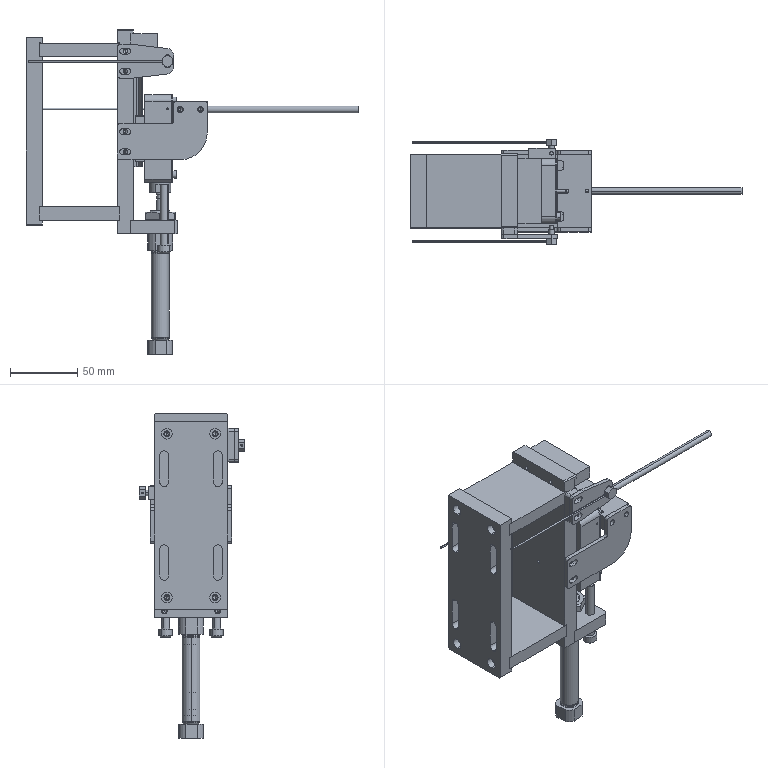Part | SolidWorks | features InContextFeatHolder 6, CompositeCurve 2 | 33 solids | 1048 faces | box 247.423 x 78.5 x 242 mm | volume 390911 mm3 | plane 517 | cylinder 375 | cone 126 | torus 14 | sphere 8 | spline 8 | commonest cylinder face diameters 3.3 x48 4 x38 2.5 x26 6 x24 4.4 x20 8 x20